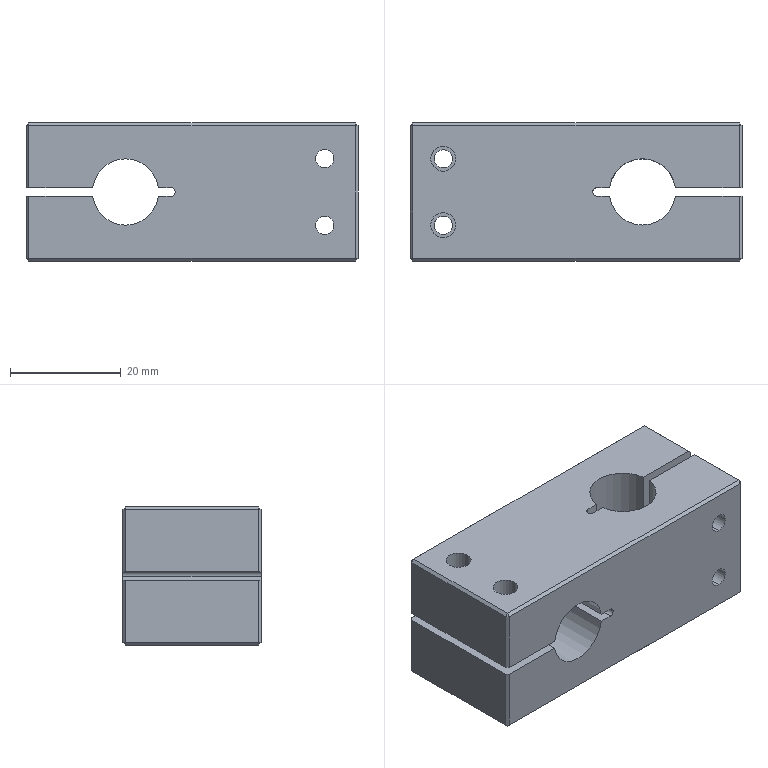Part | STEP file | ND25021-01-JDKM-36-TL | 1 solid | 65 faces | box 60 x 25 x 25 mm | volume 29527 mm3 | plane 40 | cylinder 25 | commonest cylinder face diameters 3.3 x8 4.5 x8 12 x5 1.5 x4